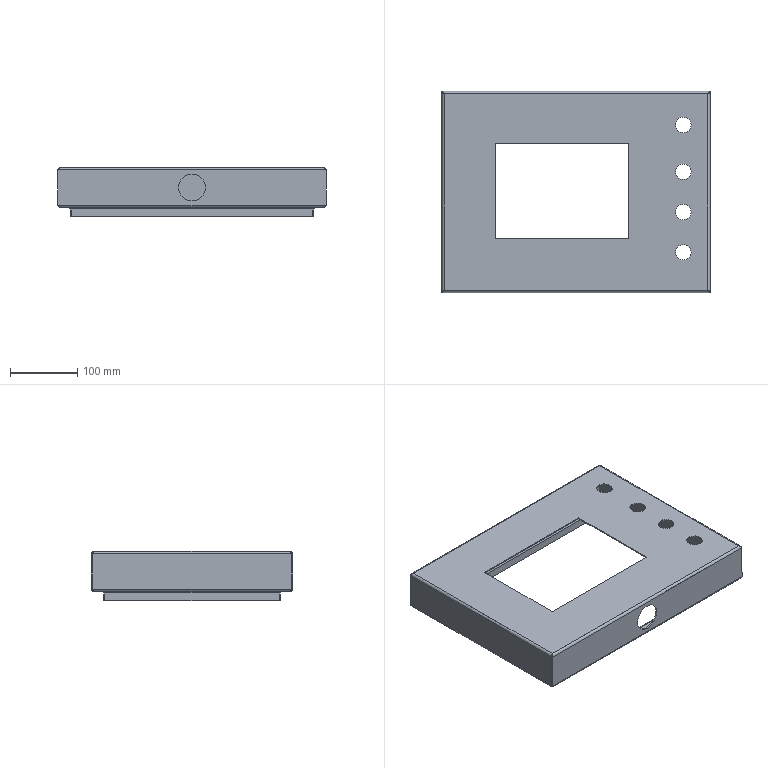Part | SolidWorks | features EdgeFlange 3, ICE 2, CornerFeat 1, FlatPattern 1, SMBaseFlange 1, SheetMetal 1 | 1 solid | 124 faces | box 400 x 300 x 73.5 mm | volume 309583 mm3 | plane 74 | cylinder 34 | spline 16 | commonest cylinder face diameters 4 x12 7 x12 23 x8 40 x2